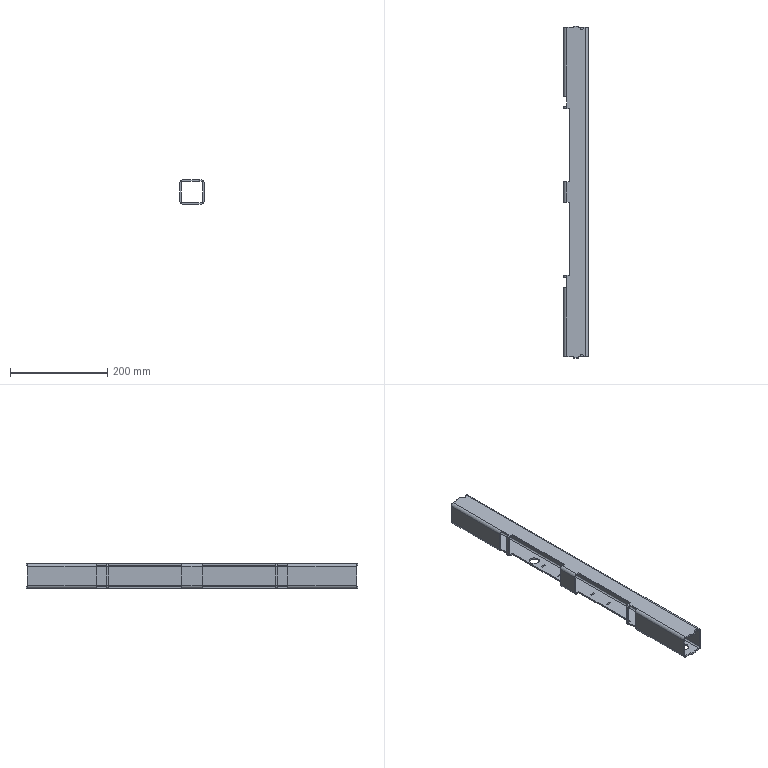Part | SolidWorks | features BaseBody 1 | 1 solid | 150 faces | box 50 x 682 x 50 mm | volume 298312 mm3 | plane 89 | cylinder 32 | spline 29 | commonest cylinder face diameters 6 x12 12 x12 20 x6 8 x2